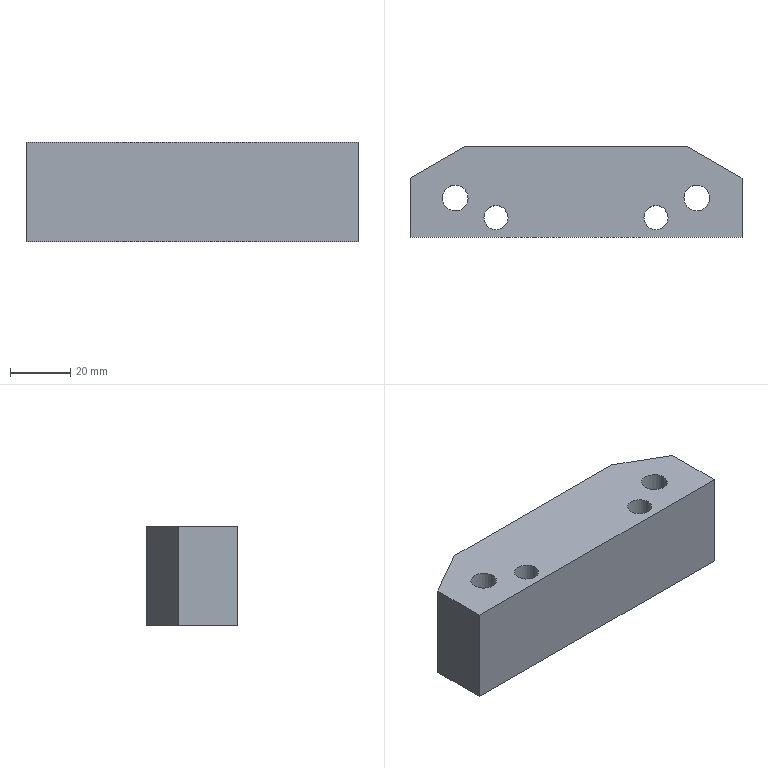Part | CATIA | 1 solid | 16 faces | box 110 x 30 x 33 mm | volume 95664 mm3 | plane 8 | cylinder 8 | commonest cylinder face diameters 8 x4 8.5 x4
STEP:
#1=CARTESIAN_POINT('',(55.,-30.,38.));
#2=VERTEX_POINT('',#1);
#3=CARTESIAN_POINT('',(55.,-30.,5.));
#4=VERTEX_POINT('',#3);
#5=CARTESIAN_POINT('',(55.,-30.,21.5));
#6=DIRECTION('',(0.,0.,-1.));
#7=VECTOR('',#6,1.);
#8=LINE('',#5,#7);
#9=EDGE_CURVE('',#2,#4,#8,.T.);
#10=ORIENTED_EDGE('',*,*,#9,.F.);
#11=CARTESIAN_POINT('',(-55.,-30.,38.));
#12=VERTEX_POINT('',#11);
#13=CARTESIAN_POINT('',(0.,-30.,38.));
#14=DIRECTION('',(-1.,0.,0.));
#15=VECTOR('',#14,1.);
#16=LINE('',#13,#15);
#17=EDGE_CURVE('',#2,#12,#16,.T.);
#18=ORIENTED_EDGE('',*,*,#17,.T.);
#19=CARTESIAN_POINT('',(-55.,-30.,5.));
#20=VERTEX_POINT('',#19);
#21=CARTESIAN_POINT('',(-55.,-30.,21.5));
#22=DIRECTION('',(0.,0.,-1.));
#23=VECTOR('',#22,1.);
#24=LINE('',#21,#23);
#25=EDGE_CURVE('',#12,#20,#24,.T.);
#26=ORIENTED_EDGE('',*,*,#25,.T.);
#27=CARTESIAN_POINT('',(0.,-30.,5.));
#28=DIRECTION('',(-1.,0.,0.));
#29=VECTOR('',#28,1.);
#30=LINE('',#27,#29);
#31=EDGE_CURVE('',#4,#20,#30,.T.);
#32=ORIENTED_EDGE('',*,*,#31,.F.);
#33=EDGE_LOOP('',(#10,#18,#26,#32));
#34=FACE_OUTER_BOUND('',#33,.T.);
#35=CARTESIAN_POINT('',(55.,-30.,38.));
#36=DIRECTION('',(0.,-1.,0.));
#37=DIRECTION('',(-1.,0.,0.));
#38=AXIS2_PLACEMENT_3D('',#35,#36,#37);
#39=PLANE('',#38);
#40=ADVANCED_FACE('',(#34),#39,.T.);
#41=CARTESIAN_POINT('',(-55.,-10.392,38.));
#42=VERTEX_POINT('',#41);
#43=CARTESIAN_POINT('',(-55.,-10.392,5.));
#44=VERTEX_POINT('',#43);
#45=CARTESIAN_POINT('',(-55.,-10.392,21.5));
#46=DIRECTION('',(0.,0.,-1.));
#47=VECTOR('',#46,1.);
#48=LINE('',#45,#47);
#49=EDGE_CURVE('',#42,#44,#48,.T.);
#50=ORIENTED_EDGE('',*,*,#49,.T.);
#51=CARTESIAN_POINT('',(-55.,-20.196,5.));
#52=DIRECTION('',(0.,-1.,0.));
#53=VECTOR('',#52,1.);
#54=LINE('',#51,#53);
#55=EDGE_CURVE('',#20,#44,#54,.F.);
#56=ORIENTED_EDGE('',*,*,#55,.F.);
#57=ORIENTED_EDGE('',*,*,#25,.F.);
#58=CARTESIAN_POINT('',(-55.,-20.196,38.));
#59=DIRECTION('',(0.,-1.,0.));
#60=VECTOR('',#59,1.);
#61=LINE('',#58,#60);
#62=EDGE_CURVE('',#12,#42,#61,.F.);
#63=ORIENTED_EDGE('',*,*,#62,.T.);
#64=EDGE_LOOP('',(#50,#56,#57,#63));
#65=FACE_OUTER_BOUND('',#64,.T.);
#66=CARTESIAN_POINT('',(-55.,0.,38.));
#67=DIRECTION('',(1.,0.,0.));
#68=DIRECTION('',(0.,-1.,0.));
#69=AXIS2_PLACEMENT_3D('',#66,#67,#68);
#70=PLANE('',#69);
#71=ADVANCED_FACE('',(#65),#70,.F.);
#72=CARTESIAN_POINT('',(-37.,0.,5.));
#73=VERTEX_POINT('',#72);
#74=CARTESIAN_POINT('',(-46.,-5.196,5.));
#75=DIRECTION('',(-0.866,-0.5,0.));
#76=VECTOR('',#75,1.);
#77=LINE('',#74,#76);
#78=EDGE_CURVE('',#73,#44,#77,.T.);
#79=ORIENTED_EDGE('',*,*,#78,.T.);
#80=ORIENTED_EDGE('',*,*,#49,.F.);
#81=CARTESIAN_POINT('',(-37.,0.,38.));
#82=VERTEX_POINT('',#81);
#83=CARTESIAN_POINT('',(-46.,-5.196,38.));
#84=DIRECTION('',(-0.866,-0.5,0.));
#85=VECTOR('',#84,1.);
#86=LINE('',#83,#85);
#87=EDGE_CURVE('',#42,#82,#86,.F.);
#88=ORIENTED_EDGE('',*,*,#87,.T.);
#89=CARTESIAN_POINT('',(-37.,0.,21.5));
#90=DIRECTION('',(0.,0.,-1.));
#91=VECTOR('',#90,1.);
#92=LINE('',#89,#91);
#93=EDGE_CURVE('',#82,#73,#92,.T.);
#94=ORIENTED_EDGE('',*,*,#93,.T.);
#95=EDGE_LOOP('',(#79,#80,#88,#94));
#96=FACE_OUTER_BOUND('',#95,.T.);
#97=CARTESIAN_POINT('',(-37.,0.,44.6));
#98=DIRECTION('',(-0.5,0.866,0.));
#99=DIRECTION('',(0.,0.,-1.));
#100=AXIS2_PLACEMENT_3D('',#97,#98,#99);
#101=PLANE('',#100);
#102=ADVANCED_FACE('',(#96),#101,.T.);
#103=CARTESIAN_POINT('',(55.,-10.392,38.));
#104=VERTEX_POINT('',#103);
#105=CARTESIAN_POINT('',(55.,-10.392,5.));
#106=VERTEX_POINT('',#105);
#107=CARTESIAN_POINT('',(55.,-10.392,21.5));
#108=DIRECTION('',(0.,0.,1.));
#109=VECTOR('',#108,1.);
#110=LINE('',#107,#109);
#111=EDGE_CURVE('',#104,#106,#110,.F.);
#112=ORIENTED_EDGE('',*,*,#111,.F.);
#113=CARTESIAN_POINT('',(55.,-20.196,38.));
#114=DIRECTION('',(0.,1.,0.));
#115=VECTOR('',#114,1.);
#116=LINE('',#113,#115);
#117=EDGE_CURVE('',#104,#2,#116,.F.);
#118=ORIENTED_EDGE('',*,*,#117,.T.);
#119=ORIENTED_EDGE('',*,*,#9,.T.);
#120=CARTESIAN_POINT('',(55.,-20.196,5.));
#121=DIRECTION('',(0.,1.,0.));
#122=VECTOR('',#121,1.);
#123=LINE('',#120,#122);
#124=EDGE_CURVE('',#106,#4,#123,.F.);
#125=ORIENTED_EDGE('',*,*,#124,.F.);
#126=EDGE_LOOP('',(#112,#118,#119,#125));
#127=FACE_OUTER_BOUND('',#126,.T.);
#128=CARTESIAN_POINT('',(55.,-30.,38.));
#129=DIRECTION('',(-1.,0.,0.));
#130=DIRECTION('',(0.,1.,0.));
#131=AXIS2_PLACEMENT_3D('',#128,#129,#130);
#132=PLANE('',#131);
#133=ADVANCED_FACE('',(#127),#132,.F.);
#134=CARTESIAN_POINT('',(37.,0.,5.));
#135=VERTEX_POINT('',#134);
#136=CARTESIAN_POINT('',(0.,0.,5.));
#137=DIRECTION('',(1.,0.,0.));
#138=VECTOR('',#137,1.);
#139=LINE('',#136,#138);
#140=EDGE_CURVE('',#73,#135,#139,.T.);
#141=ORIENTED_EDGE('',*,*,#140,.F.);
#142=ORIENTED_EDGE('',*,*,#93,.F.);
#143=CARTESIAN_POINT('',(37.,0.,38.));
#144=VERTEX_POINT('',#143);
#145=CARTESIAN_POINT('',(0.,0.,38.));
#146=DIRECTION('',(1.,0.,0.));
#147=VECTOR('',#146,1.);
#148=LINE('',#145,#147);
#149=EDGE_CURVE('',#82,#144,#148,.T.);
#150=ORIENTED_EDGE('',*,*,#149,.T.);
#151=CARTESIAN_POINT('',(37.,0.,21.5));
#152=DIRECTION('',(0.,0.,1.));
#153=VECTOR('',#152,1.);
#154=LINE('',#151,#153);
#155=EDGE_CURVE('',#144,#135,#154,.F.);
#156=ORIENTED_EDGE('',*,*,#155,.T.);
#157=EDGE_LOOP('',(#141,#142,#150,#156));
#158=FACE_OUTER_BOUND('',#157,.T.);
#159=CARTESIAN_POINT('',(-55.,0.,38.));
#160=DIRECTION('',(0.,1.,0.));
#161=DIRECTION('',(1.,0.,0.));
#162=AXIS2_PLACEMENT_3D('',#159,#160,#161);
#163=PLANE('',#162);
#164=ADVANCED_FACE('',(#158),#163,.T.);
#165=CARTESIAN_POINT('',(46.,-5.196,5.));
#166=DIRECTION('',(0.866,-0.5,0.));
#167=VECTOR('',#166,1.);
#168=LINE('',#165,#167);
#169=EDGE_CURVE('',#106,#135,#168,.F.);
#170=ORIENTED_EDGE('',*,*,#169,.T.);
#171=ORIENTED_EDGE('',*,*,#155,.F.);
#172=CARTESIAN_POINT('',(46.,-5.196,38.));
#173=DIRECTION('',(0.866,-0.5,0.));
#174=VECTOR('',#173,1.);
#175=LINE('',#172,#174);
#176=EDGE_CURVE('',#144,#104,#175,.T.);
#177=ORIENTED_EDGE('',*,*,#176,.T.);
#178=ORIENTED_EDGE('',*,*,#111,.T.);
#179=EDGE_LOOP('',(#170,#171,#177,#178));
#180=FACE_OUTER_BOUND('',#179,.T.);
#181=CARTESIAN_POINT('',(37.,0.,-1.6));
#182=DIRECTION('',(0.5,0.866,0.));
#183=DIRECTION('',(0.,0.,1.));
#184=AXIS2_PLACEMENT_3D('',#181,#182,#183);
#185=PLANE('',#184);
#186=ADVANCED_FACE('',(#180),#185,.T.);
#187=ORIENTED_EDGE('',*,*,#124,.T.);
#188=ORIENTED_EDGE('',*,*,#31,.T.);
#189=ORIENTED_EDGE('',*,*,#55,.T.);
#190=ORIENTED_EDGE('',*,*,#78,.F.);
#191=ORIENTED_EDGE('',*,*,#140,.T.);
#192=ORIENTED_EDGE('',*,*,#169,.F.);
#193=EDGE_LOOP('',(#187,#188,#189,#190,#191,#192));
#194=FACE_OUTER_BOUND('',#193,.T.);
#195=CARTESIAN_POINT('',(-43.73,-14.962,5.));
#196=VERTEX_POINT('',#195);
#197=CARTESIAN_POINT('',(-36.27,-19.038,5.));
#198=VERTEX_POINT('',#197);
#199=CARTESIAN_POINT('',(-40.,-17.,5.));
#200=DIRECTION('',(0.,0.,-1.));
#201=AXIS2_PLACEMENT_3D('',#199,#200,$);
#202=CIRCLE('',#201,4.25);
#203=EDGE_CURVE('',#196,#198,#202,.T.);
#204=ORIENTED_EDGE('',*,*,#203,.F.);
#205=CARTESIAN_POINT('',(-40.,-17.,5.));
#206=DIRECTION('',(0.,0.,-1.));
#207=AXIS2_PLACEMENT_3D('',#205,#206,$);
#208=CIRCLE('',#207,4.25);
#209=EDGE_CURVE('',#198,#196,#208,.T.);
#210=ORIENTED_EDGE('',*,*,#209,.F.);
#211=EDGE_LOOP('',(#204,#210));
#212=FACE_BOUND('',#211,.T.);
#213=CARTESIAN_POINT('',(36.27,-14.962,5.));
#214=VERTEX_POINT('',#213);
#215=CARTESIAN_POINT('',(43.73,-19.038,5.));
#216=VERTEX_POINT('',#215);
#217=CARTESIAN_POINT('',(40.,-17.,5.));
#218=DIRECTION('',(0.,0.,-1.));
#219=AXIS2_PLACEMENT_3D('',#217,#218,$);
#220=CIRCLE('',#219,4.25);
#221=EDGE_CURVE('',#214,#216,#220,.T.);
#222=ORIENTED_EDGE('',*,*,#221,.F.);
#223=CARTESIAN_POINT('',(40.,-17.,5.));
#224=DIRECTION('',(0.,0.,-1.));
#225=AXIS2_PLACEMENT_3D('',#223,#224,$);
#226=CIRCLE('',#225,4.25);
#227=EDGE_CURVE('',#216,#214,#226,.T.);
#228=ORIENTED_EDGE('',*,*,#227,.F.);
#229=EDGE_LOOP('',(#222,#228));
#230=FACE_BOUND('',#229,.T.);
#231=CARTESIAN_POINT('',(-30.01,-21.582,5.));
#232=VERTEX_POINT('',#231);
#233=CARTESIAN_POINT('',(-22.99,-25.418,5.));
#234=VERTEX_POINT('',#233);
#235=CARTESIAN_POINT('',(-26.5,-23.5,5.));
#236=DIRECTION('',(0.,0.,-1.));
#237=AXIS2_PLACEMENT_3D('',#235,#236,$);
#238=CIRCLE('',#237,4.);
#239=EDGE_CURVE('',#232,#234,#238,.T.);
#240=ORIENTED_EDGE('',*,*,#239,.F.);
#241=CARTESIAN_POINT('',(-26.5,-23.5,5.));
#242=DIRECTION('',(0.,0.,-1.));
#243=AXIS2_PLACEMENT_3D('',#241,#242,$);
#244=CIRCLE('',#243,4.);
#245=EDGE_CURVE('',#234,#232,#244,.T.);
#246=ORIENTED_EDGE('',*,*,#245,.F.);
#247=EDGE_LOOP('',(#240,#246));
#248=FACE_BOUND('',#247,.T.);
#249=CARTESIAN_POINT('',(22.99,-21.582,5.));
#250=VERTEX_POINT('',#249);
#251=CARTESIAN_POINT('',(30.01,-25.418,5.));
#252=VERTEX_POINT('',#251);
#253=CARTESIAN_POINT('',(26.5,-23.5,5.));
#254=DIRECTION('',(0.,0.,-1.));
#255=AXIS2_PLACEMENT_3D('',#253,#254,$);
#256=CIRCLE('',#255,4.);
#257=EDGE_CURVE('',#250,#252,#256,.T.);
#258=ORIENTED_EDGE('',*,*,#257,.F.);
#259=CARTESIAN_POINT('',(26.5,-23.5,5.));
#260=DIRECTION('',(0.,0.,-1.));
#261=AXIS2_PLACEMENT_3D('',#259,#260,$);
#262=CIRCLE('',#261,4.);
#263=EDGE_CURVE('',#252,#250,#262,.T.);
#264=ORIENTED_EDGE('',*,*,#263,.F.);
#265=EDGE_LOOP('',(#258,#264));
#266=FACE_BOUND('',#265,.T.);
#267=CARTESIAN_POINT('',(0.,0.,5.));
#268=DIRECTION('',(0.,0.,-1.));
#269=DIRECTION('',(1.,0.,0.));
#270=AXIS2_PLACEMENT_3D('',#267,#268,#269);
#271=PLANE('',#270);
#272=ADVANCED_FACE('',(#194,#212,#230,#248,#266),#271,.T.);
#273=ORIENTED_EDGE('',*,*,#176,.F.);
#274=ORIENTED_EDGE('',*,*,#149,.F.);
#275=ORIENTED_EDGE('',*,*,#87,.F.);
#276=ORIENTED_EDGE('',*,*,#62,.F.);
#277=ORIENTED_EDGE('',*,*,#17,.F.);
#278=ORIENTED_EDGE('',*,*,#117,.F.);
#279=EDGE_LOOP('',(#273,#274,#275,#276,#277,#278));
#280=FACE_OUTER_BOUND('',#279,.T.);
#281=CARTESIAN_POINT('',(-43.73,-14.962,38.));
#282=VERTEX_POINT('',#281);
#283=CARTESIAN_POINT('',(-36.27,-19.038,38.));
#284=VERTEX_POINT('',#283);
#285=CARTESIAN_POINT('',(-40.,-17.,38.));
#286=DIRECTION('',(0.,0.,-1.));
#287=AXIS2_PLACEMENT_3D('',#285,#286,$);
#288=CIRCLE('',#287,4.25);
#289=EDGE_CURVE('',#282,#284,#288,.T.);
#290=ORIENTED_EDGE('',*,*,#289,.T.);
#291=CARTESIAN_POINT('',(-40.,-17.,38.));
#292=DIRECTION('',(0.,0.,-1.));
#293=AXIS2_PLACEMENT_3D('',#291,#292,$);
#294=CIRCLE('',#293,4.25);
#295=EDGE_CURVE('',#284,#282,#294,.T.);
#296=ORIENTED_EDGE('',*,*,#295,.T.);
#297=EDGE_LOOP('',(#290,#296));
#298=FACE_BOUND('',#297,.T.);
#299=CARTESIAN_POINT('',(36.27,-14.962,38.));
#300=VERTEX_POINT('',#299);
#301=CARTESIAN_POINT('',(43.73,-19.038,38.));
#302=VERTEX_POINT('',#301);
#303=CARTESIAN_POINT('',(40.,-17.,38.));
#304=DIRECTION('',(0.,0.,-1.));
#305=AXIS2_PLACEMENT_3D('',#303,#304,$);
#306=CIRCLE('',#305,4.25);
#307=EDGE_CURVE('',#300,#302,#306,.T.);
#308=ORIENTED_EDGE('',*,*,#307,.T.);
#309=CARTESIAN_POINT('',(40.,-17.,38.));
#310=DIRECTION('',(0.,0.,-1.));
#311=AXIS2_PLACEMENT_3D('',#309,#310,$);
#312=CIRCLE('',#311,4.25);
#313=EDGE_CURVE('',#302,#300,#312,.T.);
#314=ORIENTED_EDGE('',*,*,#313,.T.);
#315=EDGE_LOOP('',(#308,#314));
#316=FACE_BOUND('',#315,.T.);
#317=CARTESIAN_POINT('',(-30.01,-21.582,38.));
#318=VERTEX_POINT('',#317);
#319=CARTESIAN_POINT('',(-22.99,-25.418,38.));
#320=VERTEX_POINT('',#319);
#321=CARTESIAN_POINT('',(-26.5,-23.5,38.));
#322=DIRECTION('',(0.,0.,-1.));
#323=AXIS2_PLACEMENT_3D('',#321,#322,$);
#324=CIRCLE('',#323,4.);
#325=EDGE_CURVE('',#318,#320,#324,.T.);
#326=ORIENTED_EDGE('',*,*,#325,.T.);
#327=CARTESIAN_POINT('',(-26.5,-23.5,38.));
#328=DIRECTION('',(0.,0.,-1.));
#329=AXIS2_PLACEMENT_3D('',#327,#328,$);
#330=CIRCLE('',#329,4.);
#331=EDGE_CURVE('',#320,#318,#330,.T.);
#332=ORIENTED_EDGE('',*,*,#331,.T.);
#333=EDGE_LOOP('',(#326,#332));
#334=FACE_BOUND('',#333,.T.);
#335=CARTESIAN_POINT('',(22.99,-21.582,38.));
#336=VERTEX_POINT('',#335);
#337=CARTESIAN_POINT('',(30.01,-25.418,38.));
#338=VERTEX_POINT('',#337);
#339=CARTESIAN_POINT('',(26.5,-23.5,38.));
#340=DIRECTION('',(0.,0.,-1.));
#341=AXIS2_PLACEMENT_3D('',#339,#340,$);
#342=CIRCLE('',#341,4.);
#343=EDGE_CURVE('',#336,#338,#342,.T.);
#344=ORIENTED_EDGE('',*,*,#343,.T.);
#345=CARTESIAN_POINT('',(26.5,-23.5,38.));
#346=DIRECTION('',(0.,0.,-1.));
#347=AXIS2_PLACEMENT_3D('',#345,#346,$);
#348=CIRCLE('',#347,4.);
#349=EDGE_CURVE('',#338,#336,#348,.T.);
#350=ORIENTED_EDGE('',*,*,#349,.T.);
#351=EDGE_LOOP('',(#344,#350));
#352=FACE_BOUND('',#351,.T.);
#353=CARTESIAN_POINT('',(0.,0.,38.));
#354=DIRECTION('',(0.,0.,-1.));
#355=DIRECTION('',(1.,0.,0.));
#356=AXIS2_PLACEMENT_3D('',#353,#354,#355);
#357=PLANE('',#356);
#358=ADVANCED_FACE('',(#280,#298,#316,#334,#352),#357,.F.);
#359=ORIENTED_EDGE('',*,*,#331,.F.);
#360=CARTESIAN_POINT('',(-22.99,-25.418,21.5));
#361=DIRECTION('',(0.,0.,-1.));
#362=VECTOR('',#361,1.);
#363=LINE('',#360,#362);
#364=EDGE_CURVE('',#234,#320,#363,.F.);
#365=ORIENTED_EDGE('',*,*,#364,.F.);
#366=ORIENTED_EDGE('',*,*,#245,.T.);
#367=CARTESIAN_POINT('',(-30.01,-21.582,21.5));
#368=DIRECTION('',(0.,0.,-1.));
#369=VECTOR('',#368,1.);
#370=LINE('',#367,#369);
#371=EDGE_CURVE('',#232,#318,#370,.F.);
#372=ORIENTED_EDGE('',*,*,#371,.T.);
#373=EDGE_LOOP('',(#359,#365,#366,#372));
#374=FACE_OUTER_BOUND('',#373,.T.);
#375=CARTESIAN_POINT('',(-26.5,-23.5,37.9));
#376=DIRECTION('',(0.,0.,-1.));
#377=DIRECTION('',(0.8776,-0.4794,0.));
#378=AXIS2_PLACEMENT_3D('',#375,#376,#377);
#379=CYLINDRICAL_SURFACE('',#378,4.);
#380=ADVANCED_FACE('',(#374),#379,.F.);
#381=ORIENTED_EDGE('',*,*,#325,.F.);
#382=ORIENTED_EDGE('',*,*,#371,.F.);
#383=ORIENTED_EDGE('',*,*,#239,.T.);
#384=ORIENTED_EDGE('',*,*,#364,.T.);
#385=EDGE_LOOP('',(#381,#382,#383,#384));
#386=FACE_OUTER_BOUND('',#385,.T.);
#387=ADVANCED_FACE('',(#386),#379,.F.);
#388=ORIENTED_EDGE('',*,*,#313,.F.);
#389=CARTESIAN_POINT('',(43.73,-19.038,21.5));
#390=DIRECTION('',(0.,0.,-1.));
#391=VECTOR('',#390,1.);
#392=LINE('',#389,#391);
#393=EDGE_CURVE('',#216,#302,#392,.F.);
#394=ORIENTED_EDGE('',*,*,#393,.F.);
#395=ORIENTED_EDGE('',*,*,#227,.T.);
#396=CARTESIAN_POINT('',(36.27,-14.962,21.5));
#397=DIRECTION('',(0.,0.,-1.));
#398=VECTOR('',#397,1.);
#399=LINE('',#396,#398);
#400=EDGE_CURVE('',#214,#300,#399,.F.);
#401=ORIENTED_EDGE('',*,*,#400,.T.);
#402=EDGE_LOOP('',(#388,#394,#395,#401));
#403=FACE_OUTER_BOUND('',#402,.T.);
#404=CARTESIAN_POINT('',(40.,-17.,37.9));
#405=DIRECTION('',(0.,0.,-1.));
#406=DIRECTION('',(0.8776,-0.4794,0.));
#407=AXIS2_PLACEMENT_3D('',#404,#405,#406);
#408=CYLINDRICAL_SURFACE('',#407,4.25);
#409=ADVANCED_FACE('',(#403),#408,.F.);
#410=ORIENTED_EDGE('',*,*,#307,.F.);
#411=ORIENTED_EDGE('',*,*,#400,.F.);
#412=ORIENTED_EDGE('',*,*,#221,.T.);
#413=ORIENTED_EDGE('',*,*,#393,.T.);
#414=EDGE_LOOP('',(#410,#411,#412,#413));
#415=FACE_OUTER_BOUND('',#414,.T.);
#416=ADVANCED_FACE('',(#415),#408,.F.);
#417=ORIENTED_EDGE('',*,*,#349,.F.);
#418=CARTESIAN_POINT('',(30.01,-25.418,21.5));
#419=DIRECTION('',(0.,0.,-1.));
#420=VECTOR('',#419,1.);
#421=LINE('',#418,#420);
#422=EDGE_CURVE('',#252,#338,#421,.F.);
#423=ORIENTED_EDGE('',*,*,#422,.F.);
#424=ORIENTED_EDGE('',*,*,#263,.T.);
#425=CARTESIAN_POINT('',(22.99,-21.582,21.5));
#426=DIRECTION('',(0.,0.,-1.));
#427=VECTOR('',#426,1.);
#428=LINE('',#425,#427);
#429=EDGE_CURVE('',#250,#336,#428,.F.);
#430=ORIENTED_EDGE('',*,*,#429,.T.);
#431=EDGE_LOOP('',(#417,#423,#424,#430));
#432=FACE_OUTER_BOUND('',#431,.T.);
#433=CARTESIAN_POINT('',(26.5,-23.5,37.9));
#434=DIRECTION('',(0.,0.,-1.));
#435=DIRECTION('',(0.8776,-0.4794,0.));
#436=AXIS2_PLACEMENT_3D('',#433,#434,#435);
#437=CYLINDRICAL_SURFACE('',#436,4.);
#438=ADVANCED_FACE('',(#432),#437,.F.);
#439=ORIENTED_EDGE('',*,*,#343,.F.);
#440=ORIENTED_EDGE('',*,*,#429,.F.);
#441=ORIENTED_EDGE('',*,*,#257,.T.);
#442=ORIENTED_EDGE('',*,*,#422,.T.);
#443=EDGE_LOOP('',(#439,#440,#441,#442));
#444=FACE_OUTER_BOUND('',#443,.T.);
#445=ADVANCED_FACE('',(#444),#437,.F.);
#446=ORIENTED_EDGE('',*,*,#295,.F.);
#447=CARTESIAN_POINT('',(-36.27,-19.038,21.5));
#448=DIRECTION('',(0.,0.,-1.));
#449=VECTOR('',#448,1.);
#450=LINE('',#447,#449);
#451=EDGE_CURVE('',#198,#284,#450,.F.);
#452=ORIENTED_EDGE('',*,*,#451,.F.);
#453=ORIENTED_EDGE('',*,*,#209,.T.);
#454=CARTESIAN_POINT('',(-43.73,-14.962,21.5));
#455=DIRECTION('',(0.,0.,-1.));
#456=VECTOR('',#455,1.);
#457=LINE('',#454,#456);
#458=EDGE_CURVE('',#196,#282,#457,.F.);
#459=ORIENTED_EDGE('',*,*,#458,.T.);
#460=EDGE_LOOP('',(#446,#452,#453,#459));
#461=FACE_OUTER_BOUND('',#460,.T.);
#462=CARTESIAN_POINT('',(-40.,-17.,37.9));
#463=DIRECTION('',(0.,0.,-1.));
#464=DIRECTION('',(0.8776,-0.4794,0.));
#465=AXIS2_PLACEMENT_3D('',#462,#463,#464);
#466=CYLINDRICAL_SURFACE('',#465,4.25);
#467=ADVANCED_FACE('',(#461),#466,.F.);
#468=ORIENTED_EDGE('',*,*,#289,.F.);
#469=ORIENTED_EDGE('',*,*,#458,.F.);
#470=ORIENTED_EDGE('',*,*,#203,.T.);
#471=ORIENTED_EDGE('',*,*,#451,.T.);
#472=EDGE_LOOP('',(#468,#469,#470,#471));
#473=FACE_OUTER_BOUND('',#472,.T.);
#474=ADVANCED_FACE('',(#473),#466,.F.);
#475=CLOSED_SHELL('',(#40,#71,#102,#133,#164,#186,#272,#358,#380,#387,#409,#416,#438,#445,#467,#474));
#476=MANIFOLD_SOLID_BREP('',#475);
#477=(LENGTH_UNIT()NAMED_UNIT(*)SI_UNIT(.MILLI.,.METRE.));
#478=UNCERTAINTY_MEASURE_WITH_UNIT(LENGTH_MEASURE(0.005),#477,'','');
#479=(NAMED_UNIT(*)PLANE_ANGLE_UNIT()SI_UNIT($,.RADIAN.));
#480=(NAMED_UNIT(*)SI_UNIT($,.STERADIAN.)SOLID_ANGLE_UNIT());
#481=(GEOMETRIC_REPRESENTATION_CONTEXT(3)GLOBAL_UNCERTAINTY_ASSIGNED_CONTEXT((#478))GLOBAL_UNIT_ASSIGNED_CONTEXT((#477,#479,#480))REPRESENTATION_CONTEXT('',''));
#482=ADVANCED_BREP_SHAPE_REPRESENTATION('',(#476),#481);